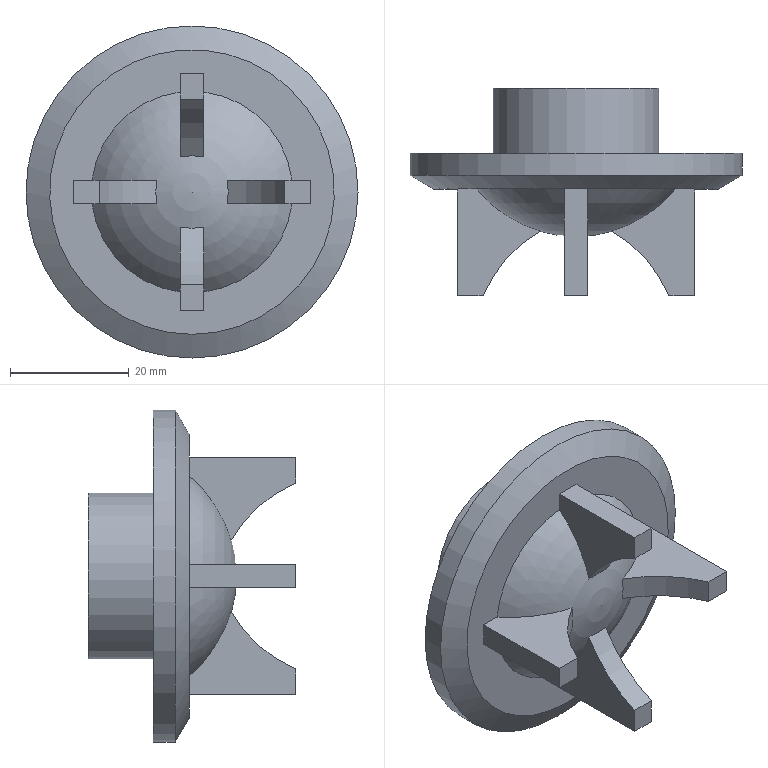Part | NX | features DATUM_CSYS 3, EXTRACT_STRING 2, EXTRUDE 2, SKETCH 2, HOLE PACKAGE 1, Instance Feature 1, Pattern Feature 1, SIMPLE HOLE 1, SWP104 1 | 1 solid | 29 faces | box 56 x 35 x 56 mm | volume 23365 mm3 | plane 19 | cylinder 7 | cone 2 | sphere 1 | commonest cylinder face diameters 46 x4 16 x1 28 x1 56 x1
STEP:
#1=CARTESIAN_POINT('',(2.,-17.,-16.852));
#2=VERTEX_POINT('',#1);
#3=CARTESIAN_POINT('',(2.,-24.075,-5.988));
#4=VERTEX_POINT('',#3);
#5=CARTESIAN_POINT('',(2.,-3.,0.));
#6=DIRECTION('',(1.,0.,0.));
#7=DIRECTION('',(0.,0.,-1.));
#8=AXIS2_PLACEMENT_3D('',#5,#6,#7);
#9=CIRCLE('',#8,21.909);
#10=EDGE_CURVE('',#2,#4,#9,.F.);
#11=ORIENTED_EDGE('',*,*,#10,.F.);
#12=CARTESIAN_POINT('',(16.852,-17.,-2.));
#13=VERTEX_POINT('',#12);
#14=CARTESIAN_POINT('',(0.,-17.,0.));
#15=DIRECTION('',(0.,-1.,0.));
#16=DIRECTION('',(0.,0.,-1.));
#17=AXIS2_PLACEMENT_3D('',#14,#15,#16);
#18=CIRCLE('',#17,16.971);
#19=EDGE_CURVE('',#2,#13,#18,.T.);
#20=ORIENTED_EDGE('',*,*,#19,.T.);
#21=CARTESIAN_POINT('',(5.988,-24.075,-2.));
#22=VERTEX_POINT('',#21);
#23=CARTESIAN_POINT('',(0.,-3.,-2.));
#24=DIRECTION('',(0.,0.,1.));
#25=DIRECTION('',(1.,0.,0.));
#26=AXIS2_PLACEMENT_3D('',#23,#24,#25);
#27=CIRCLE('',#26,21.909);
#28=EDGE_CURVE('',#13,#22,#27,.F.);
#29=ORIENTED_EDGE('',*,*,#28,.T.);
#30=CARTESIAN_POINT('',(5.988,-24.075,2.));
#31=VERTEX_POINT('',#30);
#32=CARTESIAN_POINT('',(5.988,-24.075,2.));
#33=CARTESIAN_POINT('',(6.135,-24.159,0.6667));
#34=CARTESIAN_POINT('',(6.135,-24.159,-0.6667));
#35=CARTESIAN_POINT('',(5.988,-24.075,-2.));
#36=B_SPLINE_CURVE_WITH_KNOTS('',3,(#32,#33,#34,#35),.UNSPECIFIED.,.F.,.F.,(4,4),(0.0000002,0.004),.UNSPECIFIED.);
#37=EDGE_CURVE('',#31,#22,#36,.T.);
#38=ORIENTED_EDGE('',*,*,#37,.F.);
#39=CARTESIAN_POINT('',(16.852,-17.,2.));
#40=VERTEX_POINT('',#39);
#41=CARTESIAN_POINT('',(0.,-3.,2.));
#42=DIRECTION('',(0.,0.,1.));
#43=DIRECTION('',(1.,0.,0.));
#44=AXIS2_PLACEMENT_3D('',#41,#42,#43);
#45=CIRCLE('',#44,21.909);
#46=EDGE_CURVE('',#40,#31,#45,.F.);
#47=ORIENTED_EDGE('',*,*,#46,.F.);
#48=CARTESIAN_POINT('',(2.,-17.,16.852));
#49=VERTEX_POINT('',#48);
#50=CARTESIAN_POINT('',(0.,-17.,0.));
#51=DIRECTION('',(0.,-1.,0.));
#52=DIRECTION('',(0.,0.,-1.));
#53=AXIS2_PLACEMENT_3D('',#50,#51,#52);
#54=CIRCLE('',#53,16.971);
#55=EDGE_CURVE('',#40,#49,#54,.T.);
#56=ORIENTED_EDGE('',*,*,#55,.T.);
#57=CARTESIAN_POINT('',(2.,-24.075,5.988));
#58=VERTEX_POINT('',#57);
#59=CARTESIAN_POINT('',(2.,-3.,0.));
#60=DIRECTION('',(1.,0.,0.));
#61=DIRECTION('',(0.,0.,-1.));
#62=AXIS2_PLACEMENT_3D('',#59,#60,#61);
#63=CIRCLE('',#62,21.909);
#64=EDGE_CURVE('',#58,#49,#63,.F.);
#65=ORIENTED_EDGE('',*,*,#64,.F.);
#66=CARTESIAN_POINT('',(-2.,-24.075,5.988));
#67=VERTEX_POINT('',#66);
#68=CARTESIAN_POINT('',(-2.,-24.075,5.988));
#69=CARTESIAN_POINT('',(-0.6667,-24.159,6.135));
#70=CARTESIAN_POINT('',(0.6667,-24.159,6.135));
#71=CARTESIAN_POINT('',(2.,-24.075,5.988));
#72=B_SPLINE_CURVE_WITH_KNOTS('',3,(#68,#69,#70,#71),.UNSPECIFIED.,.F.,.F.,(4,4),(0.0000002,0.004),.UNSPECIFIED.);
#73=EDGE_CURVE('',#67,#58,#72,.T.);
#74=ORIENTED_EDGE('',*,*,#73,.F.);
#75=CARTESIAN_POINT('',(-2.,-17.,16.852));
#76=VERTEX_POINT('',#75);
#77=CARTESIAN_POINT('',(-2.,-3.,0.));
#78=DIRECTION('',(1.,0.,0.));
#79=DIRECTION('',(0.,0.,-1.));
#80=AXIS2_PLACEMENT_3D('',#77,#78,#79);
#81=CIRCLE('',#80,21.909);
#82=EDGE_CURVE('',#67,#76,#81,.F.);
#83=ORIENTED_EDGE('',*,*,#82,.T.);
#84=CARTESIAN_POINT('',(-16.852,-17.,2.));
#85=VERTEX_POINT('',#84);
#86=CARTESIAN_POINT('',(0.,-17.,0.));
#87=DIRECTION('',(0.,-1.,0.));
#88=DIRECTION('',(0.,0.,-1.));
#89=AXIS2_PLACEMENT_3D('',#86,#87,#88);
#90=CIRCLE('',#89,16.971);
#91=EDGE_CURVE('',#76,#85,#90,.T.);
#92=ORIENTED_EDGE('',*,*,#91,.T.);
#93=CARTESIAN_POINT('',(-5.988,-24.075,2.));
#94=VERTEX_POINT('',#93);
#95=CARTESIAN_POINT('',(0.,-3.,2.));
#96=DIRECTION('',(0.,0.,1.));
#97=DIRECTION('',(1.,0.,0.));
#98=AXIS2_PLACEMENT_3D('',#95,#96,#97);
#99=CIRCLE('',#98,21.909);
#100=EDGE_CURVE('',#94,#85,#99,.F.);
#101=ORIENTED_EDGE('',*,*,#100,.F.);
#102=CARTESIAN_POINT('',(-5.988,-24.075,-2.));
#103=VERTEX_POINT('',#102);
#104=CARTESIAN_POINT('',(-5.988,-24.075,-2.));
#105=CARTESIAN_POINT('',(-6.135,-24.159,-0.6667));
#106=CARTESIAN_POINT('',(-6.135,-24.159,0.6667));
#107=CARTESIAN_POINT('',(-5.988,-24.075,2.));
#108=B_SPLINE_CURVE_WITH_KNOTS('',3,(#104,#105,#106,#107),.UNSPECIFIED.,.F.,.F.,(4,4),(0.0000002,0.004),.UNSPECIFIED.);
#109=EDGE_CURVE('',#103,#94,#108,.T.);
#110=ORIENTED_EDGE('',*,*,#109,.F.);
#111=CARTESIAN_POINT('',(-16.852,-17.,-2.));
#112=VERTEX_POINT('',#111);
#113=CARTESIAN_POINT('',(0.,-3.,-2.));
#114=DIRECTION('',(0.,0.,1.));
#115=DIRECTION('',(1.,0.,0.));
#116=AXIS2_PLACEMENT_3D('',#113,#114,#115);
#117=CIRCLE('',#116,21.909);
#118=EDGE_CURVE('',#103,#112,#117,.F.);
#119=ORIENTED_EDGE('',*,*,#118,.T.);
#120=CARTESIAN_POINT('',(-2.,-17.,-16.852));
#121=VERTEX_POINT('',#120);
#122=CARTESIAN_POINT('',(0.,-17.,0.));
#123=DIRECTION('',(0.,-1.,0.));
#124=DIRECTION('',(0.,0.,-1.));
#125=AXIS2_PLACEMENT_3D('',#122,#123,#124);
#126=CIRCLE('',#125,16.971);
#127=EDGE_CURVE('',#112,#121,#126,.T.);
#128=ORIENTED_EDGE('',*,*,#127,.T.);
#129=CARTESIAN_POINT('',(-2.,-24.075,-5.988));
#130=VERTEX_POINT('',#129);
#131=CARTESIAN_POINT('',(-2.,-3.,0.));
#132=DIRECTION('',(1.,0.,0.));
#133=DIRECTION('',(0.,0.,-1.));
#134=AXIS2_PLACEMENT_3D('',#131,#132,#133);
#135=CIRCLE('',#134,21.909);
#136=EDGE_CURVE('',#121,#130,#135,.F.);
#137=ORIENTED_EDGE('',*,*,#136,.T.);
#138=CARTESIAN_POINT('',(2.,-24.075,-5.988));
#139=CARTESIAN_POINT('',(0.6667,-24.159,-6.135));
#140=CARTESIAN_POINT('',(-0.6667,-24.159,-6.135));
#141=CARTESIAN_POINT('',(-2.,-24.075,-5.988));
#142=B_SPLINE_CURVE_WITH_KNOTS('',3,(#138,#139,#140,#141),.UNSPECIFIED.,.F.,.F.,(4,4),(0.0000002,0.004),.UNSPECIFIED.);
#143=EDGE_CURVE('',#4,#130,#142,.T.);
#144=ORIENTED_EDGE('',*,*,#143,.F.);
#145=EDGE_LOOP('',(#11,#20,#29,#38,#47,#56,#65,#74,#83,#92,#101,#110,#119,#128,#137,#144));
#146=FACE_BOUND('',#145,.T.);
#147=CARTESIAN_POINT('',(0.,-3.,0.));
#148=DIRECTION('',(0.,-1.,0.));
#149=DIRECTION('',(1.,0.,0.));
#150=AXIS2_PLACEMENT_3D('',#147,#148,#149);
#151=SPHERICAL_SURFACE('',#150,22.);
#152=ADVANCED_FACE('',(#146),#151,.T.);
#153=CARTESIAN_POINT('',(-2.,-17.,20.));
#154=VERTEX_POINT('',#153);
#155=CARTESIAN_POINT('',(-2.,-17.,20.));
#156=DIRECTION('',(0.,0.,-1.));
#157=VECTOR('',#156,1000.);
#158=LINE('',#155,#157);
#159=EDGE_CURVE('',#154,#76,#158,.T.);
#160=ORIENTED_EDGE('',*,*,#159,.F.);
#161=CARTESIAN_POINT('',(2.,-17.,20.));
#162=VERTEX_POINT('',#161);
#163=CARTESIAN_POINT('',(2.,-17.,20.));
#164=DIRECTION('',(-1.,0.,0.));
#165=VECTOR('',#164,1000.);
#166=LINE('',#163,#165);
#167=EDGE_CURVE('',#162,#154,#166,.T.);
#168=ORIENTED_EDGE('',*,*,#167,.F.);
#169=CARTESIAN_POINT('',(2.,-17.,20.));
#170=DIRECTION('',(0.,0.,-1.));
#171=VECTOR('',#170,1000.);
#172=LINE('',#169,#171);
#173=EDGE_CURVE('',#162,#49,#172,.T.);
#174=ORIENTED_EDGE('',*,*,#173,.T.);
#175=ORIENTED_EDGE('',*,*,#55,.F.);
#176=CARTESIAN_POINT('',(20.,-17.,2.));
#177=VERTEX_POINT('',#176);
#178=CARTESIAN_POINT('',(-20.,-17.,2.));
#179=DIRECTION('',(1.,0.,0.));
#180=VECTOR('',#179,1000.);
#181=LINE('',#178,#180);
#182=EDGE_CURVE('',#40,#177,#181,.T.);
#183=ORIENTED_EDGE('',*,*,#182,.T.);
#184=CARTESIAN_POINT('',(20.,-17.,-2.));
#185=VERTEX_POINT('',#184);
#186=CARTESIAN_POINT('',(20.,-17.,2.));
#187=DIRECTION('',(0.,0.,-1.));
#188=VECTOR('',#187,1000.);
#189=LINE('',#186,#188);
#190=EDGE_CURVE('',#177,#185,#189,.T.);
#191=ORIENTED_EDGE('',*,*,#190,.T.);
#192=CARTESIAN_POINT('',(-20.,-17.,-2.));
#193=DIRECTION('',(1.,0.,0.));
#194=VECTOR('',#193,1000.);
#195=LINE('',#192,#194);
#196=EDGE_CURVE('',#13,#185,#195,.T.);
#197=ORIENTED_EDGE('',*,*,#196,.F.);
#198=ORIENTED_EDGE('',*,*,#19,.F.);
#199=CARTESIAN_POINT('',(2.,-17.,-20.));
#200=VERTEX_POINT('',#199);
#201=CARTESIAN_POINT('',(2.,-17.,20.));
#202=DIRECTION('',(0.,0.,-1.));
#203=VECTOR('',#202,1000.);
#204=LINE('',#201,#203);
#205=EDGE_CURVE('',#2,#200,#204,.T.);
#206=ORIENTED_EDGE('',*,*,#205,.T.);
#207=CARTESIAN_POINT('',(-2.,-17.,-20.));
#208=VERTEX_POINT('',#207);
#209=CARTESIAN_POINT('',(2.,-17.,-20.));
#210=DIRECTION('',(-1.,0.,0.));
#211=VECTOR('',#210,1000.);
#212=LINE('',#209,#211);
#213=EDGE_CURVE('',#200,#208,#212,.T.);
#214=ORIENTED_EDGE('',*,*,#213,.T.);
#215=CARTESIAN_POINT('',(-2.,-17.,20.));
#216=DIRECTION('',(0.,0.,-1.));
#217=VECTOR('',#216,1000.);
#218=LINE('',#215,#217);
#219=EDGE_CURVE('',#121,#208,#218,.T.);
#220=ORIENTED_EDGE('',*,*,#219,.F.);
#221=ORIENTED_EDGE('',*,*,#127,.F.);
#222=CARTESIAN_POINT('',(-20.,-17.,-2.));
#223=VERTEX_POINT('',#222);
#224=CARTESIAN_POINT('',(-20.,-17.,-2.));
#225=DIRECTION('',(1.,0.,0.));
#226=VECTOR('',#225,1000.);
#227=LINE('',#224,#226);
#228=EDGE_CURVE('',#223,#112,#227,.T.);
#229=ORIENTED_EDGE('',*,*,#228,.F.);
#230=CARTESIAN_POINT('',(-20.,-17.,2.));
#231=VERTEX_POINT('',#230);
#232=CARTESIAN_POINT('',(-20.,-17.,2.));
#233=DIRECTION('',(0.,0.,-1.));
#234=VECTOR('',#233,1000.);
#235=LINE('',#232,#234);
#236=EDGE_CURVE('',#231,#223,#235,.T.);
#237=ORIENTED_EDGE('',*,*,#236,.F.);
#238=CARTESIAN_POINT('',(-20.,-17.,2.));
#239=DIRECTION('',(1.,0.,0.));
#240=VECTOR('',#239,1000.);
#241=LINE('',#238,#240);
#242=EDGE_CURVE('',#231,#85,#241,.T.);
#243=ORIENTED_EDGE('',*,*,#242,.T.);
#244=ORIENTED_EDGE('',*,*,#91,.F.);
#245=EDGE_LOOP('',(#160,#168,#174,#175,#183,#191,#197,#198,#206,#214,#220,#221,#229,#237,#243,#244));
#246=FACE_BOUND('',#245,.T.);
#247=CARTESIAN_POINT('',(0.,-17.,-24.));
#248=VERTEX_POINT('',#247);
#249=CARTESIAN_POINT('',(0.,-17.,0.));
#250=DIRECTION('',(0.,-1.,0.));
#251=DIRECTION('',(0.,0.,-1.));
#252=AXIS2_PLACEMENT_3D('',#249,#250,#251);
#253=CIRCLE('',#252,24.);
#254=EDGE_CURVE('',#248,#248,#253,.T.);
#255=ORIENTED_EDGE('',*,*,#254,.T.);
#256=EDGE_LOOP('',(#255));
#257=FACE_BOUND('',#256,.T.);
#258=CARTESIAN_POINT('',(16.971,-17.,0.));
#259=DIRECTION('',(0.,-1.,0.));
#260=DIRECTION('',(0.,0.,-1.));
#261=AXIS2_PLACEMENT_3D('',#258,#259,#260);
#262=PLANE('',#261);
#263=ADVANCED_FACE('',(#246,#257),#262,.T.);
#264=CARTESIAN_POINT('',(0.,-14.691,-28.));
#265=VERTEX_POINT('',#264);
#266=CARTESIAN_POINT('',(0.,-14.691,0.));
#267=DIRECTION('',(0.,-1.,0.));
#268=DIRECTION('',(0.,0.,-1.));
#269=AXIS2_PLACEMENT_3D('',#266,#267,#268);
#270=CIRCLE('',#269,28.);
#271=EDGE_CURVE('',#265,#265,#270,.T.);
#272=ORIENTED_EDGE('',*,*,#271,.T.);
#273=EDGE_LOOP('',(#272));
#274=FACE_BOUND('',#273,.T.);
#275=ORIENTED_EDGE('',*,*,#254,.F.);
#276=EDGE_LOOP('',(#275));
#277=FACE_BOUND('',#276,.T.);
#278=CARTESIAN_POINT('',(0.,-17.,0.));
#279=DIRECTION('',(0.,1.,0.));
#280=DIRECTION('',(0.,0.,1.));
#281=AXIS2_PLACEMENT_3D('',#278,#279,#280);
#282=CONICAL_SURFACE('',#281,24.,1.047);
#283=ADVANCED_FACE('',(#274,#277),#282,.T.);
#284=CARTESIAN_POINT('',(0.,-11.,-28.));
#285=VERTEX_POINT('',#284);
#286=CARTESIAN_POINT('',(0.,-11.,0.));
#287=DIRECTION('',(0.,-1.,0.));
#288=DIRECTION('',(0.,0.,-1.));
#289=AXIS2_PLACEMENT_3D('',#286,#287,#288);
#290=CIRCLE('',#289,28.);
#291=EDGE_CURVE('',#285,#285,#290,.T.);
#292=ORIENTED_EDGE('',*,*,#291,.T.);
#293=EDGE_LOOP('',(#292));
#294=FACE_BOUND('',#293,.T.);
#295=ORIENTED_EDGE('',*,*,#271,.F.);
#296=EDGE_LOOP('',(#295));
#297=FACE_BOUND('',#296,.T.);
#298=CARTESIAN_POINT('',(0.,0.,0.));
#299=DIRECTION('',(0.,-1.,0.));
#300=DIRECTION('',(0.,0.,-1.));
#301=AXIS2_PLACEMENT_3D('',#298,#299,#300);
#302=CYLINDRICAL_SURFACE('',#301,28.);
#303=ADVANCED_FACE('',(#294,#297),#302,.T.);
#304=CARTESIAN_POINT('',(0.,-11.,-14.));
#305=VERTEX_POINT('',#304);
#306=CARTESIAN_POINT('',(0.,-11.,0.));
#307=DIRECTION('',(0.,-1.,0.));
#308=DIRECTION('',(0.,0.,-1.));
#309=AXIS2_PLACEMENT_3D('',#306,#307,#308);
#310=CIRCLE('',#309,14.);
#311=EDGE_CURVE('',#305,#305,#310,.T.);
#312=ORIENTED_EDGE('',*,*,#311,.T.);
#313=EDGE_LOOP('',(#312));
#314=FACE_BOUND('',#313,.T.);
#315=ORIENTED_EDGE('',*,*,#291,.F.);
#316=EDGE_LOOP('',(#315));
#317=FACE_BOUND('',#316,.T.);
#318=CARTESIAN_POINT('',(28.,-11.,0.));
#319=DIRECTION('',(0.,1.,0.));
#320=DIRECTION('',(0.,0.,1.));
#321=AXIS2_PLACEMENT_3D('',#318,#319,#320);
#322=PLANE('',#321);
#323=ADVANCED_FACE('',(#314,#317),#322,.T.);
#324=CARTESIAN_POINT('',(0.,0.,-14.));
#325=VERTEX_POINT('',#324);
#326=CARTESIAN_POINT('',(0.,0.,0.));
#327=DIRECTION('',(0.,-1.,0.));
#328=DIRECTION('',(0.,0.,-1.));
#329=AXIS2_PLACEMENT_3D('',#326,#327,#328);
#330=CIRCLE('',#329,14.);
#331=EDGE_CURVE('',#325,#325,#330,.T.);
#332=ORIENTED_EDGE('',*,*,#331,.T.);
#333=EDGE_LOOP('',(#332));
#334=FACE_BOUND('',#333,.T.);
#335=ORIENTED_EDGE('',*,*,#311,.F.);
#336=EDGE_LOOP('',(#335));
#337=FACE_BOUND('',#336,.T.);
#338=CARTESIAN_POINT('',(0.,0.,0.));
#339=DIRECTION('',(0.,-1.,0.));
#340=DIRECTION('',(0.,0.,-1.));
#341=AXIS2_PLACEMENT_3D('',#338,#339,#340);
#342=CYLINDRICAL_SURFACE('',#341,14.);
#343=ADVANCED_FACE('',(#334,#337),#342,.T.);
#344=CARTESIAN_POINT('',(0.,0.,-8.));
#345=VERTEX_POINT('',#344);
#346=CARTESIAN_POINT('',(0.,0.,0.));
#347=DIRECTION('',(0.,-1.,0.));
#348=DIRECTION('',(0.,0.,-1.));
#349=AXIS2_PLACEMENT_3D('',#346,#347,#348);
#350=CIRCLE('',#349,8.);
#351=EDGE_CURVE('',#345,#345,#350,.T.);
#352=ORIENTED_EDGE('',*,*,#351,.T.);
#353=EDGE_LOOP('',(#352));
#354=FACE_BOUND('',#353,.T.);
#355=ORIENTED_EDGE('',*,*,#331,.F.);
#356=EDGE_LOOP('',(#355));
#357=FACE_BOUND('',#356,.T.);
#358=CARTESIAN_POINT('',(14.,0.,0.));
#359=DIRECTION('',(0.,1.,0.));
#360=DIRECTION('',(0.,0.,1.));
#361=AXIS2_PLACEMENT_3D('',#358,#359,#360);
#362=PLANE('',#361);
#363=ADVANCED_FACE('',(#354,#357),#362,.T.);
#364=CARTESIAN_POINT('',(20.,-35.,-2.));
#365=VERTEX_POINT('',#364);
#366=CARTESIAN_POINT('',(15.666,-35.,-2.));
#367=VERTEX_POINT('',#366);
#368=CARTESIAN_POINT('',(20.,-35.,-2.));
#369=DIRECTION('',(-1.,0.,0.));
#370=VECTOR('',#369,1000.);
#371=LINE('',#368,#370);
#372=EDGE_CURVE('',#365,#367,#371,.T.);
#373=ORIENTED_EDGE('',*,*,#372,.F.);
#374=CARTESIAN_POINT('',(20.,-35.,2.));
#375=VERTEX_POINT('',#374);
#376=CARTESIAN_POINT('',(20.,-35.,2.));
#377=DIRECTION('',(0.,0.,-1.));
#378=VECTOR('',#377,1000.);
#379=LINE('',#376,#378);
#380=EDGE_CURVE('',#375,#365,#379,.T.);
#381=ORIENTED_EDGE('',*,*,#380,.F.);
#382=CARTESIAN_POINT('',(15.666,-35.,2.));
#383=VERTEX_POINT('',#382);
#384=CARTESIAN_POINT('',(20.,-35.,2.));
#385=DIRECTION('',(-1.,0.,0.));
#386=VECTOR('',#385,1000.);
#387=LINE('',#384,#386);
#388=EDGE_CURVE('',#375,#383,#387,.T.);
#389=ORIENTED_EDGE('',*,*,#388,.T.);
#390=CARTESIAN_POINT('',(15.666,-35.,2.));
#391=DIRECTION('',(0.,0.,-1.));
#392=VECTOR('',#391,1000.);
#393=LINE('',#390,#392);
#394=EDGE_CURVE('',#383,#367,#393,.T.);
#395=ORIENTED_EDGE('',*,*,#394,.T.);
#396=EDGE_LOOP('',(#373,#381,#389,#395));
#397=FACE_BOUND('',#396,.T.);
#398=CARTESIAN_POINT('',(20.,-35.,2.));
#399=DIRECTION('',(0.,-1.,0.));
#400=DIRECTION('',(0.,0.,-1.));
#401=AXIS2_PLACEMENT_3D('',#398,#399,#400);
#402=PLANE('',#401);
#403=ADVANCED_FACE('',(#397),#402,.T.);
#404=CARTESIAN_POINT('',(20.,-17.,-2.));
#405=DIRECTION('',(0.,-1.,0.));
#406=VECTOR('',#405,1000.);
#407=LINE('',#404,#406);
#408=EDGE_CURVE('',#185,#365,#407,.T.);
#409=ORIENTED_EDGE('',*,*,#408,.F.);
#410=ORIENTED_EDGE('',*,*,#190,.F.);
#411=CARTESIAN_POINT('',(20.,-17.,2.));
#412=DIRECTION('',(0.,-1.,0.));
#413=VECTOR('',#412,1000.);
#414=LINE('',#411,#413);
#415=EDGE_CURVE('',#177,#375,#414,.T.);
#416=ORIENTED_EDGE('',*,*,#415,.T.);
#417=ORIENTED_EDGE('',*,*,#380,.T.);
#418=EDGE_LOOP('',(#409,#410,#416,#417));
#419=FACE_BOUND('',#418,.T.);
#420=CARTESIAN_POINT('',(20.,-17.,2.));
#421=DIRECTION('',(1.,0.,0.));
#422=DIRECTION('',(0.,0.,-1.));
#423=AXIS2_PLACEMENT_3D('',#420,#421,#422);
#424=PLANE('',#423);
#425=ADVANCED_FACE('',(#419),#424,.T.);
#426=ORIENTED_EDGE('',*,*,#28,.F.);
#427=ORIENTED_EDGE('',*,*,#196,.T.);
#428=ORIENTED_EDGE('',*,*,#408,.T.);
#429=ORIENTED_EDGE('',*,*,#372,.T.);
#430=CARTESIAN_POINT('',(-5.5,-44.,-2.));
#431=DIRECTION('',(0.,0.,1.));
#432=DIRECTION('',(1.,0.,0.));
#433=AXIS2_PLACEMENT_3D('',#430,#431,#432);
#434=CIRCLE('',#433,23.);
#435=EDGE_CURVE('',#367,#22,#434,.T.);
#436=ORIENTED_EDGE('',*,*,#435,.T.);
#437=EDGE_LOOP('',(#426,#427,#428,#429,#436));
#438=FACE_BOUND('',#437,.T.);
#439=CARTESIAN_POINT('',(-5.5,-44.,-2.));
#440=DIRECTION('',(0.,0.,1.));
#441=DIRECTION('',(1.,0.,0.));
#442=AXIS2_PLACEMENT_3D('',#439,#440,#441);
#443=PLANE('',#442);
#444=ADVANCED_FACE('',(#438),#443,.F.);
#445=ORIENTED_EDGE('',*,*,#182,.F.);
#446=ORIENTED_EDGE('',*,*,#46,.T.);
#447=CARTESIAN_POINT('',(-5.5,-44.,2.));
#448=DIRECTION('',(0.,0.,1.));
#449=DIRECTION('',(1.,0.,0.));
#450=AXIS2_PLACEMENT_3D('',#447,#448,#449);
#451=CIRCLE('',#450,23.);
#452=EDGE_CURVE('',#383,#31,#451,.T.);
#453=ORIENTED_EDGE('',*,*,#452,.F.);
#454=ORIENTED_EDGE('',*,*,#388,.F.);
#455=ORIENTED_EDGE('',*,*,#415,.F.);
#456=EDGE_LOOP('',(#445,#446,#453,#454,#455));
#457=FACE_BOUND('',#456,.T.);
#458=CARTESIAN_POINT('',(-5.5,-44.,2.));
#459=DIRECTION('',(0.,0.,1.));
#460=DIRECTION('',(1.,0.,0.));
#461=AXIS2_PLACEMENT_3D('',#458,#459,#460);
#462=PLANE('',#461);
#463=ADVANCED_FACE('',(#457),#462,.T.);
#464=ORIENTED_EDGE('',*,*,#452,.T.);
#465=ORIENTED_EDGE('',*,*,#37,.T.);
#466=ORIENTED_EDGE('',*,*,#435,.F.);
#467=ORIENTED_EDGE('',*,*,#394,.F.);
#468=EDGE_LOOP('',(#464,#465,#466,#467));
#469=FACE_BOUND('',#468,.T.);
#470=CARTESIAN_POINT('',(-5.5,-44.,2.));
#471=DIRECTION('',(0.,0.,-1.));
#472=DIRECTION('',(-1.,0.,0.));
#473=AXIS2_PLACEMENT_3D('',#470,#471,#472);
#474=CYLINDRICAL_SURFACE('',#473,23.);
#475=ADVANCED_FACE('',(#469),#474,.F.);
#476=CARTESIAN_POINT('',(-20.,-35.,-2.));
#477=VERTEX_POINT('',#476);
#478=CARTESIAN_POINT('',(-20.,-35.,-2.));
#479=DIRECTION('',(0.,1.,0.));
#480=VECTOR('',#479,1000.);
#481=LINE('',#478,#480);
#482=EDGE_CURVE('',#477,#223,#481,.T.);
#483=ORIENTED_EDGE('',*,*,#482,.F.);
#484=CARTESIAN_POINT('',(-20.,-35.,2.));
#485=VERTEX_POINT('',#484);
#486=CARTESIAN_POINT('',(-20.,-35.,2.));
#487=DIRECTION('',(0.,0.,-1.));
#488=VECTOR('',#487,1000.);
#489=LINE('',#486,#488);
#490=EDGE_CURVE('',#485,#477,#489,.T.);
#491=ORIENTED_EDGE('',*,*,#490,.F.);
#492=CARTESIAN_POINT('',(-20.,-35.,2.));
#493=DIRECTION('',(0.,1.,0.));
#494=VECTOR('',#493,1000.);
#495=LINE('',#492,#494);
#496=EDGE_CURVE('',#485,#231,#495,.T.);
#497=ORIENTED_EDGE('',*,*,#496,.T.);
#498=ORIENTED_EDGE('',*,*,#236,.T.);
#499=EDGE_LOOP('',(#483,#491,#497,#498));
#500=FACE_BOUND('',#499,.T.);
#501=CARTESIAN_POINT('',(-20.,-35.,2.));
#502=DIRECTION('',(-1.,0.,0.));
#503=DIRECTION('',(0.,0.,1.));
#504=AXIS2_PLACEMENT_3D('',#501,#502,#503);
#505=PLANE('',#504);
#506=ADVANCED_FACE('',(#500),#505,.T.);
#507=CARTESIAN_POINT('',(-15.666,-35.,-2.));
#508=VERTEX_POINT('',#507);
#509=CARTESIAN_POINT('',(5.5,-44.,-2.));
#510=DIRECTION('',(0.,0.,1.));
#511=DIRECTION('',(1.,0.,0.));
#512=AXIS2_PLACEMENT_3D('',#509,#510,#511);
#513=CIRCLE('',#512,23.);
#514=EDGE_CURVE('',#103,#508,#513,.T.);
#515=ORIENTED_EDGE('',*,*,#514,.F.);
#516=ORIENTED_EDGE('',*,*,#109,.T.);
#517=CARTESIAN_POINT('',(-15.666,-35.,2.));
#518=VERTEX_POINT('',#517);
#519=CARTESIAN_POINT('',(5.5,-44.,2.));
#520=DIRECTION('',(0.,0.,1.));
#521=DIRECTION('',(1.,0.,0.));
#522=AXIS2_PLACEMENT_3D('',#519,#520,#521);
#523=CIRCLE('',#522,23.);
#524=EDGE_CURVE('',#94,#518,#523,.T.);
#525=ORIENTED_EDGE('',*,*,#524,.T.);
#526=CARTESIAN_POINT('',(-15.666,-35.,2.));
#527=DIRECTION('',(0.,0.,-1.));
#528=VECTOR('',#527,1000.);
#529=LINE('',#526,#528);
#530=EDGE_CURVE('',#518,#508,#529,.T.);
#531=ORIENTED_EDGE('',*,*,#530,.T.);
#532=EDGE_LOOP('',(#515,#516,#525,#531));
#533=FACE_BOUND('',#532,.T.);
#534=CARTESIAN_POINT('',(5.5,-44.,2.));
#535=DIRECTION('',(0.,0.,-1.));
#536=DIRECTION('',(-1.,0.,0.));
#537=AXIS2_PLACEMENT_3D('',#534,#535,#536);
#538=CYLINDRICAL_SURFACE('',#537,23.);
#539=ADVANCED_FACE('',(#533),#538,.F.);
#540=CARTESIAN_POINT('',(-15.666,-35.,-2.));
#541=DIRECTION('',(-1.,0.,0.));
#542=VECTOR('',#541,1000.);
#543=LINE('',#540,#542);
#544=EDGE_CURVE('',#508,#477,#543,.T.);
#545=ORIENTED_EDGE('',*,*,#544,.F.);
#546=ORIENTED_EDGE('',*,*,#530,.F.);
#547=CARTESIAN_POINT('',(-15.666,-35.,2.));
#548=DIRECTION('',(-1.,0.,0.));
#549=VECTOR('',#548,1000.);
#550=LINE('',#547,#549);
#551=EDGE_CURVE('',#518,#485,#550,.T.);
#552=ORIENTED_EDGE('',*,*,#551,.T.);
#553=ORIENTED_EDGE('',*,*,#490,.T.);
#554=EDGE_LOOP('',(#545,#546,#552,#553));
#555=FACE_BOUND('',#554,.T.);
#556=CARTESIAN_POINT('',(-15.666,-35.,2.));
#557=DIRECTION('',(0.,-1.,0.));
#558=DIRECTION('',(0.,0.,-1.));
#559=AXIS2_PLACEMENT_3D('',#556,#557,#558);
#560=PLANE('',#559);
#561=ADVANCED_FACE('',(#555),#560,.T.);
#562=ORIENTED_EDGE('',*,*,#524,.F.);
#563=ORIENTED_EDGE('',*,*,#100,.T.);
#564=ORIENTED_EDGE('',*,*,#242,.F.);
#565=ORIENTED_EDGE('',*,*,#496,.F.);
#566=ORIENTED_EDGE('',*,*,#551,.F.);
#567=EDGE_LOOP('',(#562,#563,#564,#565,#566));
#568=FACE_BOUND('',#567,.T.);
#569=CARTESIAN_POINT('',(-5.5,-44.,2.));
#570=DIRECTION('',(0.,0.,1.));
#571=DIRECTION('',(1.,0.,0.));
#572=AXIS2_PLACEMENT_3D('',#569,#570,#571);
#573=PLANE('',#572);
#574=ADVANCED_FACE('',(#568),#573,.T.);
#575=ORIENTED_EDGE('',*,*,#118,.F.);
#576=ORIENTED_EDGE('',*,*,#514,.T.);
#577=ORIENTED_EDGE('',*,*,#544,.T.);
#578=ORIENTED_EDGE('',*,*,#482,.T.);
#579=ORIENTED_EDGE('',*,*,#228,.T.);
#580=EDGE_LOOP('',(#575,#576,#577,#578,#579));
#581=FACE_BOUND('',#580,.T.);
#582=CARTESIAN_POINT('',(-5.5,-44.,-2.));
#583=DIRECTION('',(0.,0.,1.));
#584=DIRECTION('',(1.,0.,0.));
#585=AXIS2_PLACEMENT_3D('',#582,#583,#584);
#586=PLANE('',#585);
#587=ADVANCED_FACE('',(#581),#586,.F.);
#588=CARTESIAN_POINT('',(-2.,-35.,-20.));
#589=VERTEX_POINT('',#588);
#590=CARTESIAN_POINT('',(-2.,-35.,-15.666));
#591=VERTEX_POINT('',#590);
#592=CARTESIAN_POINT('',(-2.,-35.,-20.));
#593=DIRECTION('',(0.,0.,1.));
#594=VECTOR('',#593,1000.);
#595=LINE('',#592,#594);
#596=EDGE_CURVE('',#589,#591,#595,.T.);
#597=ORIENTED_EDGE('',*,*,#596,.F.);
#598=CARTESIAN_POINT('',(2.,-35.,-20.));
#599=VERTEX_POINT('',#598);
#600=CARTESIAN_POINT('',(2.,-35.,-20.));
#601=DIRECTION('',(-1.,0.,0.));
#602=VECTOR('',#601,1000.);
#603=LINE('',#600,#602);
#604=EDGE_CURVE('',#599,#589,#603,.T.);
#605=ORIENTED_EDGE('',*,*,#604,.F.);
#606=CARTESIAN_POINT('',(2.,-35.,-15.666));
#607=VERTEX_POINT('',#606);
#608=CARTESIAN_POINT('',(2.,-35.,-20.));
#609=DIRECTION('',(0.,0.,1.));
#610=VECTOR('',#609,1000.);
#611=LINE('',#608,#610);
#612=EDGE_CURVE('',#599,#607,#611,.T.);
#613=ORIENTED_EDGE('',*,*,#612,.T.);
#614=CARTESIAN_POINT('',(2.,-35.,-15.666));
#615=DIRECTION('',(-1.,0.,0.));
#616=VECTOR('',#615,1000.);
#617=LINE('',#614,#616);
#618=EDGE_CURVE('',#607,#591,#617,.T.);
#619=ORIENTED_EDGE('',*,*,#618,.T.);
#620=EDGE_LOOP('',(#597,#605,#613,#619));
#621=FACE_BOUND('',#620,.T.);
#622=CARTESIAN_POINT('',(2.,-35.,-20.));
#623=DIRECTION('',(0.,-1.,0.));
#624=DIRECTION('',(0.,0.,-1.));
#625=AXIS2_PLACEMENT_3D('',#622,#623,#624);
#626=PLANE('',#625);
#627=ADVANCED_FACE('',(#621),#626,.T.);
#628=CARTESIAN_POINT('',(-2.,-17.,-20.));
#629=DIRECTION('',(0.,-1.,0.));
#630=VECTOR('',#629,1000.);
#631=LINE('',#628,#630);
#632=EDGE_CURVE('',#208,#589,#631,.T.);
#633=ORIENTED_EDGE('',*,*,#632,.F.);
#634=ORIENTED_EDGE('',*,*,#213,.F.);
#635=CARTESIAN_POINT('',(2.,-17.,-20.));
#636=DIRECTION('',(0.,-1.,0.));
#637=VECTOR('',#636,1000.);
#638=LINE('',#635,#637);
#639=EDGE_CURVE('',#200,#599,#638,.T.);
#640=ORIENTED_EDGE('',*,*,#639,.T.);
#641=ORIENTED_EDGE('',*,*,#604,.T.);
#642=EDGE_LOOP('',(#633,#634,#640,#641));
#643=FACE_BOUND('',#642,.T.);
#644=CARTESIAN_POINT('',(2.,-17.,-20.));
#645=DIRECTION('',(0.,0.,-1.));
#646=DIRECTION('',(-1.,0.,0.));
#647=AXIS2_PLACEMENT_3D('',#644,#645,#646);
#648=PLANE('',#647);
#649=ADVANCED_FACE('',(#643),#648,.T.);
#650=ORIENTED_EDGE('',*,*,#136,.F.);
#651=ORIENTED_EDGE('',*,*,#219,.T.);
#652=ORIENTED_EDGE('',*,*,#632,.T.);
#653=ORIENTED_EDGE('',*,*,#596,.T.);
#654=CARTESIAN_POINT('',(-2.,-44.,5.5));
#655=DIRECTION('',(1.,0.,0.));
#656=DIRECTION('',(0.,0.,-1.));
#657=AXIS2_PLACEMENT_3D('',#654,#655,#656);
#658=CIRCLE('',#657,23.);
#659=EDGE_CURVE('',#591,#130,#658,.T.);
#660=ORIENTED_EDGE('',*,*,#659,.T.);
#661=EDGE_LOOP('',(#650,#651,#652,#653,#660));
#662=FACE_BOUND('',#661,.T.);
#663=CARTESIAN_POINT('',(-2.,-44.,5.5));
#664=DIRECTION('',(1.,0.,0.));
#665=DIRECTION('',(0.,0.,-1.));
#666=AXIS2_PLACEMENT_3D('',#663,#664,#665);
#667=PLANE('',#666);
#668=ADVANCED_FACE('',(#662),#667,.F.);
#669=ORIENTED_EDGE('',*,*,#205,.F.);
#670=ORIENTED_EDGE('',*,*,#10,.T.);
#671=CARTESIAN_POINT('',(2.,-44.,5.5));
#672=DIRECTION('',(1.,0.,0.));
#673=DIRECTION('',(0.,0.,-1.));
#674=AXIS2_PLACEMENT_3D('',#671,#672,#673);
#675=CIRCLE('',#674,23.);
#676=EDGE_CURVE('',#607,#4,#675,.T.);
#677=ORIENTED_EDGE('',*,*,#676,.F.);
#678=ORIENTED_EDGE('',*,*,#612,.F.);
#679=ORIENTED_EDGE('',*,*,#639,.F.);
#680=EDGE_LOOP('',(#669,#670,#677,#678,#679));
#681=FACE_BOUND('',#680,.T.);
#682=CARTESIAN_POINT('',(2.,-44.,5.5));
#683=DIRECTION('',(1.,0.,0.));
#684=DIRECTION('',(0.,0.,-1.));
#685=AXIS2_PLACEMENT_3D('',#682,#683,#684);
#686=PLANE('',#685);
#687=ADVANCED_FACE('',(#681),#686,.T.);
#688=ORIENTED_EDGE('',*,*,#676,.T.);
#689=ORIENTED_EDGE('',*,*,#143,.T.);
#690=ORIENTED_EDGE('',*,*,#659,.F.);
#691=ORIENTED_EDGE('',*,*,#618,.F.);
#692=EDGE_LOOP('',(#688,#689,#690,#691));
#693=FACE_BOUND('',#692,.T.);
#694=CARTESIAN_POINT('',(2.,-44.,5.5));
#695=DIRECTION('',(-1.,0.,0.));
#696=DIRECTION('',(0.,0.,1.));
#697=AXIS2_PLACEMENT_3D('',#694,#695,#696);
#698=CYLINDRICAL_SURFACE('',#697,23.);
#699=ADVANCED_FACE('',(#693),#698,.F.);
#700=CARTESIAN_POINT('',(-2.,-35.,20.));
#701=VERTEX_POINT('',#700);
#702=CARTESIAN_POINT('',(-2.,-35.,20.));
#703=DIRECTION('',(0.,1.,0.));
#704=VECTOR('',#703,1000.);
#705=LINE('',#702,#704);
#706=EDGE_CURVE('',#701,#154,#705,.T.);
#707=ORIENTED_EDGE('',*,*,#706,.F.);
#708=CARTESIAN_POINT('',(2.,-35.,20.));
#709=VERTEX_POINT('',#708);
#710=CARTESIAN_POINT('',(2.,-35.,20.));
#711=DIRECTION('',(-1.,0.,0.));
#712=VECTOR('',#711,1000.);
#713=LINE('',#710,#712);
#714=EDGE_CURVE('',#709,#701,#713,.T.);
#715=ORIENTED_EDGE('',*,*,#714,.F.);
#716=CARTESIAN_POINT('',(2.,-35.,20.));
#717=DIRECTION('',(0.,1.,0.));
#718=VECTOR('',#717,1000.);
#719=LINE('',#716,#718);
#720=EDGE_CURVE('',#709,#162,#719,.T.);
#721=ORIENTED_EDGE('',*,*,#720,.T.);
#722=ORIENTED_EDGE('',*,*,#167,.T.);
#723=EDGE_LOOP('',(#707,#715,#721,#722));
#724=FACE_BOUND('',#723,.T.);
#725=CARTESIAN_POINT('',(2.,-35.,20.));
#726=DIRECTION('',(0.,0.,1.));
#727=DIRECTION('',(1.,0.,0.));
#728=AXIS2_PLACEMENT_3D('',#725,#726,#727);
#729=PLANE('',#728);
#730=ADVANCED_FACE('',(#724),#729,.T.);
#731=CARTESIAN_POINT('',(-2.,-35.,15.666));
#732=VERTEX_POINT('',#731);
#733=CARTESIAN_POINT('',(-2.,-44.,-5.5));
#734=DIRECTION('',(1.,0.,0.));
#735=DIRECTION('',(0.,0.,-1.));
#736=AXIS2_PLACEMENT_3D('',#733,#734,#735);
#737=CIRCLE('',#736,23.);
#738=EDGE_CURVE('',#67,#732,#737,.T.);
#739=ORIENTED_EDGE('',*,*,#738,.F.);
#740=ORIENTED_EDGE('',*,*,#73,.T.);
#741=CARTESIAN_POINT('',(2.,-35.,15.666));
#742=VERTEX_POINT('',#741);
#743=CARTESIAN_POINT('',(2.,-44.,-5.5));
#744=DIRECTION('',(1.,0.,0.));
#745=DIRECTION('',(0.,0.,-1.));
#746=AXIS2_PLACEMENT_3D('',#743,#744,#745);
#747=CIRCLE('',#746,23.);
#748=EDGE_CURVE('',#58,#742,#747,.T.);
#749=ORIENTED_EDGE('',*,*,#748,.T.);
#750=CARTESIAN_POINT('',(2.,-35.,15.666));
#751=DIRECTION('',(-1.,0.,0.));
#752=VECTOR('',#751,1000.);
#753=LINE('',#750,#752);
#754=EDGE_CURVE('',#742,#732,#753,.T.);
#755=ORIENTED_EDGE('',*,*,#754,.T.);
#756=EDGE_LOOP('',(#739,#740,#749,#755));
#757=FACE_BOUND('',#756,.T.);
#758=CARTESIAN_POINT('',(2.,-44.,-5.5));
#759=DIRECTION('',(-1.,0.,0.));
#760=DIRECTION('',(0.,0.,1.));
#761=AXIS2_PLACEMENT_3D('',#758,#759,#760);
#762=CYLINDRICAL_SURFACE('',#761,23.);
#763=ADVANCED_FACE('',(#757),#762,.F.);
#764=CARTESIAN_POINT('',(-2.,-35.,15.666));
#765=DIRECTION('',(0.,0.,1.));
#766=VECTOR('',#765,1000.);
#767=LINE('',#764,#766);
#768=EDGE_CURVE('',#732,#701,#767,.T.);
#769=ORIENTED_EDGE('',*,*,#768,.F.);
#770=ORIENTED_EDGE('',*,*,#754,.F.);
#771=CARTESIAN_POINT('',(2.,-35.,15.666));
#772=DIRECTION('',(0.,0.,1.));
#773=VECTOR('',#772,1000.);
#774=LINE('',#771,#773);
#775=EDGE_CURVE('',#742,#709,#774,.T.);
#776=ORIENTED_EDGE('',*,*,#775,.T.);
#777=ORIENTED_EDGE('',*,*,#714,.T.);
#778=EDGE_LOOP('',(#769,#770,#776,#777));
#779=FACE_BOUND('',#778,.T.);
#780=CARTESIAN_POINT('',(2.,-35.,15.666));
#781=DIRECTION('',(0.,-1.,0.));
#782=DIRECTION('',(0.,0.,-1.));
#783=AXIS2_PLACEMENT_3D('',#780,#781,#782);
#784=PLANE('',#783);
#785=ADVANCED_FACE('',(#779),#784,.T.);
#786=ORIENTED_EDGE('',*,*,#748,.F.);
#787=ORIENTED_EDGE('',*,*,#64,.T.);
#788=ORIENTED_EDGE('',*,*,#173,.F.);
#789=ORIENTED_EDGE('',*,*,#720,.F.);
#790=ORIENTED_EDGE('',*,*,#775,.F.);
#791=EDGE_LOOP('',(#786,#787,#788,#789,#790));
#792=FACE_BOUND('',#791,.T.);
#793=CARTESIAN_POINT('',(2.,-44.,5.5));
#794=DIRECTION('',(1.,0.,0.));
#795=DIRECTION('',(0.,0.,-1.));
#796=AXIS2_PLACEMENT_3D('',#793,#794,#795);
#797=PLANE('',#796);
#798=ADVANCED_FACE('',(#792),#797,.T.);
#799=ORIENTED_EDGE('',*,*,#82,.F.);
#800=ORIENTED_EDGE('',*,*,#738,.T.);
#801=ORIENTED_EDGE('',*,*,#768,.T.);
#802=ORIENTED_EDGE('',*,*,#706,.T.);
#803=ORIENTED_EDGE('',*,*,#159,.T.);
#804=EDGE_LOOP('',(#799,#800,#801,#802,#803));
#805=FACE_BOUND('',#804,.T.);
#806=CARTESIAN_POINT('',(-2.,-44.,5.5));
#807=DIRECTION('',(1.,0.,0.));
#808=DIRECTION('',(0.,0.,-1.));
#809=AXIS2_PLACEMENT_3D('',#806,#807,#808);
#810=PLANE('',#809);
#811=ADVANCED_FACE('',(#805),#810,.F.);
#812=CARTESIAN_POINT('',(0.,-16.,-8.));
#813=VERTEX_POINT('',#812);
#814=CARTESIAN_POINT('',(0.,-16.,0.));
#815=DIRECTION('',(0.,-1.,0.));
#816=DIRECTION('',(0.,0.,-1.));
#817=AXIS2_PLACEMENT_3D('',#814,#815,#816);
#818=CIRCLE('',#817,8.);
#819=EDGE_CURVE('',#813,#813,#818,.F.);
#820=ORIENTED_EDGE('',*,*,#819,.T.);
#821=EDGE_LOOP('',(#820));
#822=FACE_BOUND('',#821,.T.);
#823=CARTESIAN_POINT('',(0.,-20.807,0.));
#824=VERTEX_POINT('',#823);
#825=VERTEX_LOOP('',#824);
#826=FACE_BOUND('',#825,.T.);
#827=CARTESIAN_POINT('',(0.,-16.,0.));
#828=DIRECTION('',(0.,1.,0.));
#829=DIRECTION('',(0.,0.,1.));
#830=AXIS2_PLACEMENT_3D('',#827,#828,#829);
#831=CONICAL_SURFACE('',#830,8.,1.03);
#832=ADVANCED_FACE('',(#822,#826),#831,.F.);
#833=ORIENTED_EDGE('',*,*,#819,.F.);
#834=EDGE_LOOP('',(#833));
#835=FACE_BOUND('',#834,.T.);
#836=ORIENTED_EDGE('',*,*,#351,.F.);
#837=EDGE_LOOP('',(#836));
#838=FACE_BOUND('',#837,.T.);
#839=CARTESIAN_POINT('',(0.,0.,0.));
#840=DIRECTION('',(0.,-1.,0.));
#841=DIRECTION('',(0.,0.,-1.));
#842=AXIS2_PLACEMENT_3D('',#839,#840,#841);
#843=CYLINDRICAL_SURFACE('',#842,8.);
#844=ADVANCED_FACE('',(#835,#838),#843,.F.);
#845=CLOSED_SHELL('',(#152,#263,#283,#303,#323,#343,#363,#403,#425,#444,#463,#475,#506,#539,#561,#574,#587,#627,#649,#668,#687,#699,#730,#763,#785,#798,#811,#832,#844));
#846=MANIFOLD_SOLID_BREP('',#845);
#847=(LENGTH_UNIT()NAMED_UNIT(*)SI_UNIT(.MILLI.,.METRE.));
#848=UNCERTAINTY_MEASURE_WITH_UNIT(LENGTH_MEASURE(0.0508),#847,'','');
#849=(NAMED_UNIT(*)PLANE_ANGLE_UNIT()SI_UNIT($,.RADIAN.));
#850=(NAMED_UNIT(*)SI_UNIT($,.STERADIAN.)SOLID_ANGLE_UNIT());
#851=(GEOMETRIC_REPRESENTATION_CONTEXT(3)GLOBAL_UNCERTAINTY_ASSIGNED_CONTEXT((#848))GLOBAL_UNIT_ASSIGNED_CONTEXT((#847,#849,#850))REPRESENTATION_CONTEXT('',''));
#852=ADVANCED_BREP_SHAPE_REPRESENTATION('',(#846),#851);